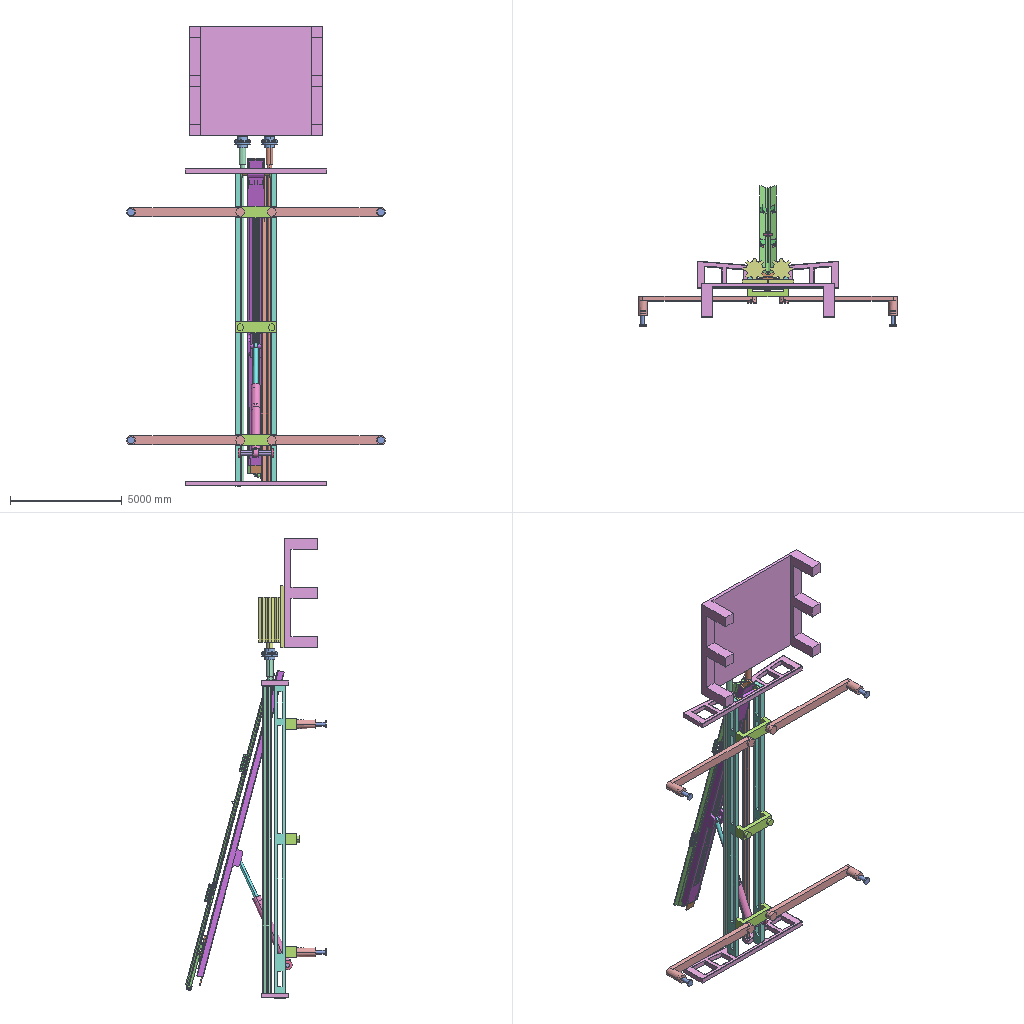Assembly | SolidWorks | 33 different items | 69 placed | box 11606 x 6308 x 20604 mm
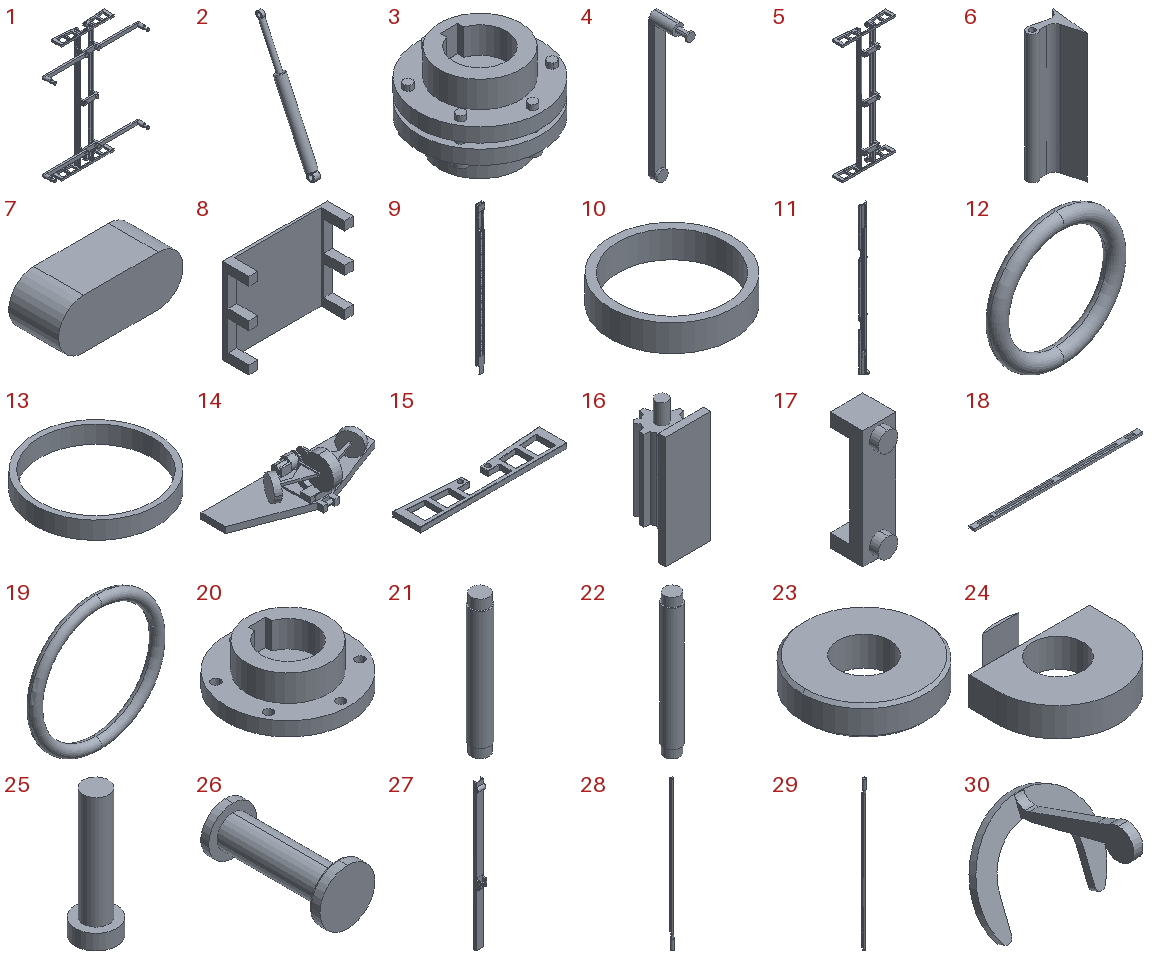Parts list (item | name | quantity | parent item | size | volume | features):
1 | (subassembly) | x1 | - | 11606 x 2886 x 14220 mm | 6344611681 mm3 | features ReferencePattern 2, MirrorCompFeat 1
2 | (subassembly) | x1 | - | 400 x 2533 x 5104 mm | 258998356 mm3 | -
3 | (subassembly) | x2 | - | 700 x 700 x 490 mm | 90960757 mm3 | features ReferencePattern 5, CompositeCurve 1, LocalCirPattern 1
4 | (subassembly) | x4 | in 1 | 400 x 1336 x 5303 mm | 513861042 mm3 | features CompositeCurve 2, AEMSimFeature 1
5 | (subassembly) | x1 | in 1 | 6350 x 1686 x 14220 mm | 4157610963 mm3 | -
6 | - | x4 | - | 210.318 x 232.159 x 790 mm | 10438808 mm3 | features Fillet 2, Extrusion 1
7 | - | x2 | - | 250 x 100 x 100 mm | 2285398 mm3 | features Extrusion 1
8 | - | x1 | - | 6000 x 1500 x 4914 mm | 6959700000 mm3 | features Extrusion 1, ICE 1
9 | - | x1 | - | 600 x 410.622 x 14546 mm | 1021826260 mm3 | features ICE 18, Extrusion 1
10 | - | x1 | in 2 | 230 x 230 x 50 mm | 506582 mm3 | features Extrusion 1
11 | - | x1 | - | 771.866 x 352.673 x 14699 mm | 861943756 mm3 | features ICE 41, Extrusion 1
12 | - | x1 | in 2 | 250 x 30 x 250 mm | 488545 mm3 | features RefAxis 1, Revolution 1
13 | - | x2 | - | 350 x 350 x 50 mm | 814419 mm3 | features Extrusion 1
14 | - | x1 | - | 393.785 x 164.433 x 118.113 mm | 975900 mm3 | features ICE 20, Fillet 5, Extrusion 1
15 | - | x2 | in 5 | 6350 x 1200 x 220 mm | 732765661 mm3 | features Fillet 8, ICE 3, Cut 2, Extrusion 1
16 | - | x2 | - | 1126 x 1145 x 3030 mm | 1733566944 mm3 | features ICE 5, Extrusion 1
17 | - | x3 | in 5 | 500 x 636 x 1800 mm | 259226547 mm3 | features ICE 2, Extrusion 1
18 | - | x2 | in 5 | 14220 x 500 x 200 mm | 957200000 mm3 | features ICE 2, Extrusion 1
19 | - | x1 | - | 360 x 30 x 360 mm | 732818 mm3 | features RefAxis 1, Revolution 1
20 | - | x4 | in 3 | 700 x 700 x 230 mm | 43732082 mm3 | features ICE 2, Extrusion 1
21 | - | x1 | in 1 | 200 x 200 x 1400 mm | 42509676 mm3 | features Extrusion 1, ICE 1
22 | - | x1 | in 1 | 200 x 200 x 1600 mm | 48792861 mm3 | features Extrusion 1, ICE 1
23 | - | x2 | in 1 | 420 x 420 x 100 mm | 11319289 mm3 | features Chamfer 1, Extrusion 1
24 | - | x2 | in 1 | 420 x 420 x 100 mm | 8807720 mm3 | features ICE 2, Extrusion 1
25 | - | x12 | in 3 | 80 x 80 x 250 mm | 582765 mm3 | features Extrusion 1, ICE 1
26 | - | x4 | in 4 | 316.364 x 705 x 316.364 mm | 22636383 mm3 | features ICE 2, Extrusion 1, Fillet 1
27 | - | x1 | - | 750 x 589 x 14150 mm | 669271540 mm3 | features ICE 11, Fillet 2, Extrusion 1
28 | - | x1 | - | 300 x 474.612 x 15314 mm | 388904585 mm3 | features ICE 9, Extrusion 1
29 | - | x1 | - | 300 x 474.612 x 15244 mm | 386924782 mm3 | features ICE 6, Extrusion 1
30 | - | x1 | - | 200 x 205.934 x 192.17 mm | 208238 mm3 | features ICE 2, Extrusion 1, Fillet 1
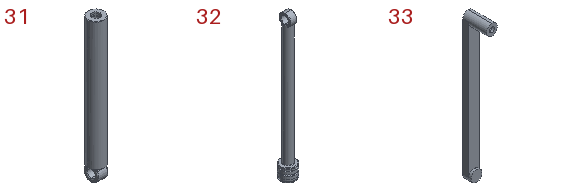31 | - | x1 | in 2 | 400 x 400 x 3541 mm | 139018402 mm3 | features ICE 10, Fillet 3, RevCut 2, Chamfer 1, Extrusion 1
32 | - | x1 | in 2 | 349 x 349 x 3335 mm | 118986511 mm3 | features ICE 4, Fillet 2, RevCut 2, Extrusion 1
33 | - | x4 | in 4 | 400 x 866 x 5303 mm | 491224658 mm3 | features ICE 5, Extrusion 1
Mates (type | each side: item.copy, entity, surface, feature):
In the top assembly
Width | 15.1 face plane Boss-Extrude1 | 15.1 face plane Boss-Extrude1 | 8.1 face plane Boss-Extrude1 | 8.1 face plane Boss-Extrude1
Concentric | 15.2 face cylinder Cut-Extrude2 | 28.1 face cylinder Boss-Extrude1
Coincident | 15.2 face plane Boss-Extrude1 | 28.1 face plane Cut-Extrude1
Concentric | 15.2 face cylinder Cut-Extrude2 | 29.1 face cylinder Boss-Extrude3
Coincident | 15.2 face plane Boss-Extrude1 | 29.1 face plane Boss-Extrude2
Parallel | 26.1 face plane Boss-Extrude3 | 8.1 face plane Boss-Extrude1
Width | 15.1 face plane Cut-Extrude5 | 15.1 face plane Cut-Extrude5 | 27.1 face plane Boss-Extrude3 | 27.1 face plane Boss-Extrude3
Concentric | 22.1 face cylinder Boss-Extrude1 | 31.1 face cylinder Boss-Extrude7
Concentric | 21.1 face cylinder Boss-Extrude1 | 27.1 face cylinder Cut-Extrude3
Concentric | 20.1 face cylinder Boss-Extrude1 | 16.1 face cylinder Boss-Extrude1
Coincident | 8.1 face plane Boss-Extrude1 | 16.1 face plane Boss-Extrude4
DistanceDim | 16.1 face plane Cut-Extrude2 | 20.1 face plane Boss-Extrude1
Coincident | 16.1 face plane Boss-Extrude4 | 16.2 face plane Boss-Extrude4
Coincident | 27.1 face plane Boss-Extrude1 | 9.1 face plane Boss-Extrude2 | 3 times
Concentric | 32.1 face cylinder Cut-Extrude1 | 27.1 face cylinder Boss-Extrude5
Parallel | 28.1 face plane Cut-Extrude3 | 7.1 face plane Boss-Extrude1
Coincident | 28.1 face plane Cut-Extrude3 | 7.1 face plane Boss-Extrude1 | 2 times
Concentric | 28.1 face cylinder Boss-Extrude7 | 20.2 face cylinder Boss-Extrude1
Coincident | 29.1 face plane Boss-Extrude6 | 7.2 face plane Boss-Extrude1
Coincident | 29.1 face plane Cut-Extrude2 | 7.2 face plane Boss-Extrude1
Concentric | 29.1 face cylinder Boss-Extrude5 | 20.3 face cylinder Boss-Extrude1
Coincident | 29.1 face plane Boss-Extrude5 | 20.3 face plane Boss-Extrude2
Coincident | 14.1 face plane Cut-Extrude1 | 30.1 face plane Boss-Extrude1
Concentric | 14.1 face cylinder Boss-Extrude8 | 30.1 face cylinder Boss-Extrude1
Coincident | 14.1 edge | 30.1 face plane Boss-Extrude2
Concentric | 32.1 face cylinder Boss-Extrude2 | 19.1 axis
Symmetric | 32.1 face plane Cut-Revolve3 | 32.1 face plane Cut-Revolve3 | 19.1 plane
Concentric | 32.1 face cylinder Cut-Revolve1 | 13.1 face cylinder Boss-Extrude1
Coincident | 32.1 face plane Cut-Revolve1 | 13.1 face plane Boss-Extrude1
Concentric | 32.1 face cylinder Cut-Revolve1 | 13.2 face cylinder Boss-Extrude1
Coincident | 32.1 face plane Cut-Revolve1 | 13.2 face plane Boss-Extrude1
Coincident | 11.1 axis | 6.1 axis
Coincident | 11.1 face plane Cut-Extrude10 | 6.1 face plane Boss-Extrude1
Concentric | 11.1 face cylinder Boss-Extrude18 | 6.2 face cylinder Boss-Extrude1
Coincident | 11.1 face plane Cut-Extrude10 | 6.2 face plane Boss-Extrude1
Concentric | 11.1 face cylinder Boss-Extrude17 | 6.3 face cylinder Boss-Extrude1
Coincident | 11.1 face plane Cut-Extrude10 | 6.3 face plane Boss-Extrude1
Concentric | 11.1 face cylinder Boss-Extrude17 | 6.4 face cylinder Boss-Extrude1
Coincident | 11.1 face plane Cut-Extrude10 | 6.4 face plane Boss-Extrude1
Parallel | 20.3 face plane Boss-Extrude1 | 7.2 face plane Boss-Extrude1
Coincident | 8.1 face plane Boss-Extrude1 | 16.2 face plane Boss-Extrude4 | 2 times
Concentric | 9.1 face cylinder Cut-Extrude2 | 11.1 face cylinder Boss-Extrude29
Coincident | 9.1 face plane Cut-Extrude3 | 11.1 face plane Cut-Extrude2
Parallel | 9.1 face plane Boss-Extrude2 | 11.1 face plane Cut-Extrude6
Coincident | 11.1 face plane Cut-Extrude6 | 14.1 face plane Boss-Extrude1
Tangent | 11.1 face plane Cut-Extrude6 | 14.1 face cylinder Boss-Extrude1
Parallel | 11.1 face plane Cut-Extrude6 | 14.1 face plane Boss-Extrude17
Parallel | 7.1 face plane Boss-Extrude1 | 20.2 face plane Boss-Extrude1
Concentric | 16.2 face cylinder Boss-Extrude1 | 20.4 face cylinder Boss-Extrude1
Concentric | 29.1 face cylinder Cut-Extrude2 | 7.2 face cylinder Boss-Extrude1
Coincident | 20.1 face plane Boss-Extrude1 | 20.4 face plane Boss-Extrude1
Concentric | 28.1 face cylinder Cut-Extrude3 | 7.1 face cylinder Boss-Extrude1
In subassembly 1
Parallel | 18.1 face plane Boss-Extrude1 | 1.1 plane
Coincident | 18.1 face plane Boss-Extrude1 | 23.1 face plane Boss-Extrude1
Tangent | 18.1 face plane Boss-Extrude1 | 23.1 face cylinder Boss-Extrude1 | 2 times
Concentric | 23.1 face cylinder Boss-Extrude1 | 23.2 face cylinder Boss-Extrude1
Coincident | 18.2 face plane Boss-Extrude1 | 23.2 face plane Boss-Extrude1
Concentric | 23.1 face cylinder Boss-Extrude1 | 21.2 face cylinder Boss-Extrude1
Coincident | 18.1 face plane Boss-Extrude1 | 21.2 face plane Boss-Extrude1
Coincident | 18.2 face plane Boss-Extrude1 | 24.1 face plane Boss-Extrude2
Coincident | 18.2 face plane Boss-Extrude1 | 24.1 face plane Boss-Extrude1
Coincident | 18.1 face plane Boss-Extrude1 | 24.2 face plane Boss-Extrude2
Coincident | 18.1 face plane Boss-Extrude1 | 24.2 face plane Boss-Extrude1
Concentric | 24.2 face cylinder Boss-Extrude1 | 22.2 face cylinder Boss-Extrude1
Concentric | 24.1 face cylinder Boss-Extrude1 | 22.2 face cylinder Boss-Extrude1
Coincident | 24.1 face plane Boss-Extrude1 | 22.2 face plane Boss-Extrude1
DistanceDim | 24.2 face plane Boss-Extrude2 | 17.1 face plane Boss-Extrude1
Concentric | 17.2 face cylinder Boss-Extrude2 | 33.1 face cylinder Boss-Extrude1
Coincident | 17.2 face plane Boss-Extrude1 | 33.1 face plane Boss-Extrude1
Concentric | 17.1 face cylinder Boss-Extrude2 | 33.2 face cylinder Boss-Extrude1
Coincident | 17.1 face plane Boss-Extrude1 | 33.2 face plane Boss-Extrude1
Parallel | 17.1 face plane Boss-Extrude1 | 33.2 face plane Boss-Extrude2
In subassembly 4
Concentric | 33.3 edge | 26.2 edge
LimitDistanceDim | 26.2 face plane Boss-Extrude1 | 33.3 face plane Cut-Extrude1
In subassembly 5
Width | 15.3 face plane Boss-Extrude1 | 15.3 face plane Boss-Extrude1 | 18.3 face plane Boss-Extrude1 | 18.4 face plane Boss-Extrude1
Coincident | 15.4 face plane Boss-Extrude1 | 15.3 face plane Boss-Extrude1 | 2 times
Coincident | 18.4 face plane Boss-Extrude1 | 17.3 face plane Boss-Extrude1 | 2 times
Coincident | 18.3 face plane Boss-Extrude1 | 17.3 face plane Boss-Extrude1 | 2 times
Coincident | 17.4 face plane Boss-Extrude1 | 18.4 face plane Boss-Extrude1 | 2 times
DistanceDim | 18.4 face plane Boss-Extrude1 | 15.3 face plane Boss-Extrude1
Coincident | 15.3 face plane Boss-Extrude1 | 18.4 face plane Boss-Extrude1
Coincident | 15.4 face plane Boss-Extrude1 | 18.4 face plane Boss-Extrude1
Coincident | 18.3 face plane Boss-Extrude1 | 15.4 face plane Boss-Extrude1
Coincident | 18.3 face plane Cut-Extrude1 | 17.3 face plane Boss-Extrude1
Coincident | 18.4 face plane Boss-Extrude1 | 17.5 face plane Boss-Extrude1 | 2 times
Coincident | 18.4 face plane Cut-Extrude1 | 17.5 face plane Boss-Extrude1
DistanceDim | 17.4 face plane Boss-Extrude1 | 18.3 face plane Cut-Extrude1
In subassembly 2
Symmetric | 31.2 face plane Cut-Revolve1 | 31.2 face plane Cut-Revolve1 | 12.1 plane
Coincident | 31.2 face plane Cut-Revolve2 | 10.1 face plane Boss-Extrude1
Concentric | 31.2 face cylinder Boss-Extrude2 | 32.2 face cylinder Boss-Extrude2
Concentric | 32.2 face cylinder Boss-Extrude2 | 12.1 axis
Concentric | 32.2 face cylinder Boss-Extrude2 | 10.1 face cylinder Boss-Extrude1
In subassembly 3
Concentric | 20.5 edge | 20.6 face cylinder Cut-Extrude1
Concentric | 20.5 face cylinder Cut-Extrude1 | 20.6 face cylinder Cut-Extrude1
Concentric | 20.5 face cylinder Cut-Extrude1 | 25.1 face cylinder Boss-Extrude1
Coincident | 20.5 face plane Boss-Extrude2 | 25.1 face plane Boss-Extrude2
DistanceDim | 20.5 face plane Boss-Extrude2 | 20.6 face plane Boss-Extrude2